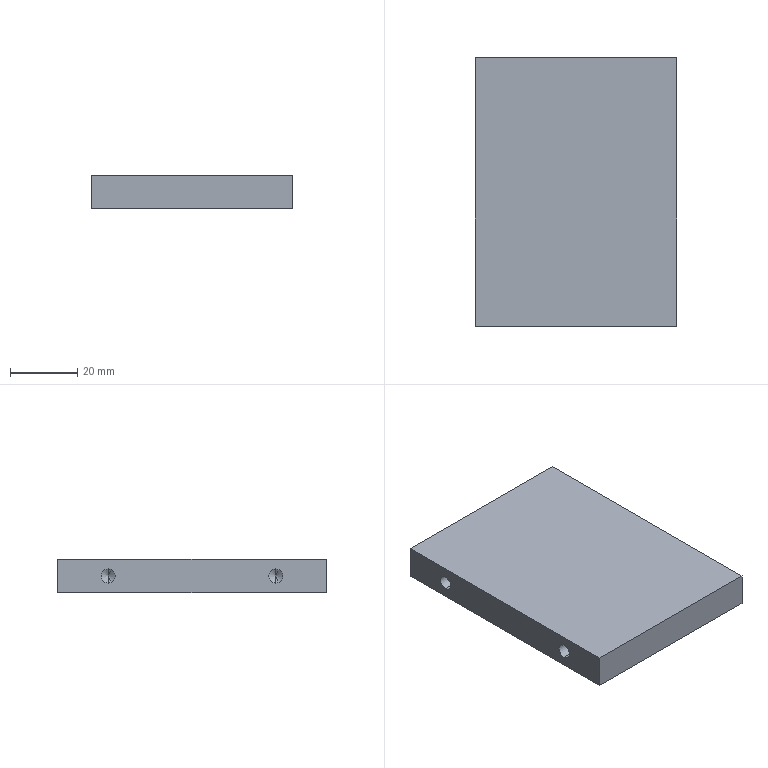Part | SolidWorks | features HoleWzd 2, Extrusion 1 | 1 solid | 22 faces | box 60 x 80 x 10 mm | volume 47201 mm3 | cylinder 8 | cone 8 | plane 6 | commonest cylinder face diameters 4.2 x8
STEP:
#1=CARTESIAN_POINT('',(-16.,25.,2.9));
#2=VERTEX_POINT('',#1);
#3=CARTESIAN_POINT('',(-16.,25.,7.1));
#4=VERTEX_POINT('',#3);
#5=CARTESIAN_POINT('',(-16.,25.,5.));
#6=DIRECTION('',(-1.,0.,0.));
#7=DIRECTION('',(0.,0.,1.));
#8=AXIS2_PLACEMENT_3D('',#5,#6,#7);
#9=CIRCLE('',#8,2.1);
#10=EDGE_CURVE('',#2,#4,#9,.T.);
#11=ORIENTED_EDGE('',*,*,#10,.F.);
#12=CARTESIAN_POINT('',(-30.,25.,2.9));
#13=VERTEX_POINT('',#12);
#14=CARTESIAN_POINT('',(-30.,25.,2.9));
#15=DIRECTION('',(-1.,0.,0.));
#16=VECTOR('',#15,1000.);
#17=LINE('',#14,#16);
#18=EDGE_CURVE('',#2,#13,#17,.T.);
#19=ORIENTED_EDGE('',*,*,#18,.T.);
#20=CARTESIAN_POINT('',(-30.,25.,7.1));
#21=VERTEX_POINT('',#20);
#22=CARTESIAN_POINT('',(-30.,25.,5.));
#23=DIRECTION('',(-1.,0.,0.));
#24=DIRECTION('',(0.,0.,1.));
#25=AXIS2_PLACEMENT_3D('',#22,#23,#24);
#26=CIRCLE('',#25,2.1);
#27=EDGE_CURVE('',#13,#21,#26,.T.);
#28=ORIENTED_EDGE('',*,*,#27,.T.);
#29=CARTESIAN_POINT('',(-30.,25.,7.1));
#30=DIRECTION('',(-1.,0.,0.));
#31=VECTOR('',#30,1000.);
#32=LINE('',#29,#31);
#33=EDGE_CURVE('',#4,#21,#32,.T.);
#34=ORIENTED_EDGE('',*,*,#33,.F.);
#35=EDGE_LOOP('',(#11,#19,#28,#34));
#36=FACE_OUTER_BOUND('',#35,.T.);
#37=CARTESIAN_POINT('',(-30.,25.,5.));
#38=DIRECTION('',(-1.,0.,0.));
#39=DIRECTION('',(0.,0.,1.));
#40=AXIS2_PLACEMENT_3D('',#37,#38,#39);
#41=CYLINDRICAL_SURFACE('',#40,2.1);
#42=ADVANCED_FACE('',(#36),#41,.F.);
#43=CARTESIAN_POINT('',(-14.738,25.,5.));
#44=VERTEX_POINT('',#43);
#45=CARTESIAN_POINT('',(-16.,25.,7.1));
#46=DIRECTION('',(-0.515,0.,0.8572));
#47=VECTOR('',#46,1000.);
#48=LINE('',#45,#47);
#49=EDGE_CURVE('',#44,#4,#48,.T.);
#50=ORIENTED_EDGE('',*,*,#49,.F.);
#51=CARTESIAN_POINT('',(-16.,25.,2.9));
#52=DIRECTION('',(-0.515,0.,-0.8572));
#53=VECTOR('',#52,1000.);
#54=LINE('',#51,#53);
#55=EDGE_CURVE('',#44,#2,#54,.T.);
#56=ORIENTED_EDGE('',*,*,#55,.T.);
#57=ORIENTED_EDGE('',*,*,#10,.T.);
#58=EDGE_LOOP('',(#50,#56,#57));
#59=FACE_OUTER_BOUND('',#58,.T.);
#60=CARTESIAN_POINT('',(-16.,25.,5.));
#61=DIRECTION('',(-1.,0.,0.));
#62=DIRECTION('',(0.,0.,1.));
#63=AXIS2_PLACEMENT_3D('',#60,#61,#62);
#64=CONICAL_SURFACE('',#63,2.1,1.03);
#65=ADVANCED_FACE('',(#59),#64,.F.);
#66=CARTESIAN_POINT('',(-16.,-25.,2.9));
#67=VERTEX_POINT('',#66);
#68=CARTESIAN_POINT('',(-16.,-25.,7.1));
#69=VERTEX_POINT('',#68);
#70=CARTESIAN_POINT('',(-16.,-25.,5.));
#71=DIRECTION('',(-1.,0.,0.));
#72=DIRECTION('',(0.,0.,1.));
#73=AXIS2_PLACEMENT_3D('',#70,#71,#72);
#74=CIRCLE('',#73,2.1);
#75=EDGE_CURVE('',#67,#69,#74,.T.);
#76=ORIENTED_EDGE('',*,*,#75,.F.);
#77=CARTESIAN_POINT('',(-30.,-25.,2.9));
#78=VERTEX_POINT('',#77);
#79=CARTESIAN_POINT('',(-30.,-25.,2.9));
#80=DIRECTION('',(-1.,0.,0.));
#81=VECTOR('',#80,1000.);
#82=LINE('',#79,#81);
#83=EDGE_CURVE('',#67,#78,#82,.T.);
#84=ORIENTED_EDGE('',*,*,#83,.T.);
#85=CARTESIAN_POINT('',(-30.,-25.,7.1));
#86=VERTEX_POINT('',#85);
#87=CARTESIAN_POINT('',(-30.,-25.,5.));
#88=DIRECTION('',(-1.,0.,0.));
#89=DIRECTION('',(0.,0.,1.));
#90=AXIS2_PLACEMENT_3D('',#87,#88,#89);
#91=CIRCLE('',#90,2.1);
#92=EDGE_CURVE('',#78,#86,#91,.T.);
#93=ORIENTED_EDGE('',*,*,#92,.T.);
#94=CARTESIAN_POINT('',(-30.,-25.,7.1));
#95=DIRECTION('',(-1.,0.,0.));
#96=VECTOR('',#95,1000.);
#97=LINE('',#94,#96);
#98=EDGE_CURVE('',#69,#86,#97,.T.);
#99=ORIENTED_EDGE('',*,*,#98,.F.);
#100=EDGE_LOOP('',(#76,#84,#93,#99));
#101=FACE_OUTER_BOUND('',#100,.T.);
#102=CARTESIAN_POINT('',(-30.,-25.,5.));
#103=DIRECTION('',(-1.,0.,0.));
#104=DIRECTION('',(0.,0.,1.));
#105=AXIS2_PLACEMENT_3D('',#102,#103,#104);
#106=CYLINDRICAL_SURFACE('',#105,2.1);
#107=ADVANCED_FACE('',(#101),#106,.F.);
#108=CARTESIAN_POINT('',(-14.738,-25.,5.));
#109=VERTEX_POINT('',#108);
#110=CARTESIAN_POINT('',(-16.,-25.,7.1));
#111=DIRECTION('',(-0.515,0.,0.8572));
#112=VECTOR('',#111,1000.);
#113=LINE('',#110,#112);
#114=EDGE_CURVE('',#109,#69,#113,.T.);
#115=ORIENTED_EDGE('',*,*,#114,.F.);
#116=CARTESIAN_POINT('',(-16.,-25.,2.9));
#117=DIRECTION('',(-0.515,0.,-0.8572));
#118=VECTOR('',#117,1000.);
#119=LINE('',#116,#118);
#120=EDGE_CURVE('',#109,#67,#119,.T.);
#121=ORIENTED_EDGE('',*,*,#120,.T.);
#122=ORIENTED_EDGE('',*,*,#75,.T.);
#123=EDGE_LOOP('',(#115,#121,#122));
#124=FACE_OUTER_BOUND('',#123,.T.);
#125=CARTESIAN_POINT('',(-16.,-25.,5.));
#126=DIRECTION('',(-1.,0.,0.));
#127=DIRECTION('',(0.,0.,1.));
#128=AXIS2_PLACEMENT_3D('',#125,#126,#127);
#129=CONICAL_SURFACE('',#128,2.1,1.03);
#130=ADVANCED_FACE('',(#124),#129,.F.);
#131=CARTESIAN_POINT('',(16.,-25.,7.1));
#132=VERTEX_POINT('',#131);
#133=CARTESIAN_POINT('',(16.,-25.,2.9));
#134=VERTEX_POINT('',#133);
#135=CARTESIAN_POINT('',(16.,-25.,5.));
#136=DIRECTION('',(1.,0.,0.));
#137=DIRECTION('',(0.,0.,-1.));
#138=AXIS2_PLACEMENT_3D('',#135,#136,#137);
#139=CIRCLE('',#138,2.1);
#140=EDGE_CURVE('',#132,#134,#139,.T.);
#141=ORIENTED_EDGE('',*,*,#140,.F.);
#142=CARTESIAN_POINT('',(30.,-25.,7.1));
#143=VERTEX_POINT('',#142);
#144=CARTESIAN_POINT('',(30.,-25.,7.1));
#145=DIRECTION('',(1.,0.,0.));
#146=VECTOR('',#145,1000.);
#147=LINE('',#144,#146);
#148=EDGE_CURVE('',#132,#143,#147,.T.);
#149=ORIENTED_EDGE('',*,*,#148,.T.);
#150=CARTESIAN_POINT('',(30.,-25.,2.9));
#151=VERTEX_POINT('',#150);
#152=CARTESIAN_POINT('',(30.,-25.,5.));
#153=DIRECTION('',(1.,0.,0.));
#154=DIRECTION('',(0.,0.,-1.));
#155=AXIS2_PLACEMENT_3D('',#152,#153,#154);
#156=CIRCLE('',#155,2.1);
#157=EDGE_CURVE('',#143,#151,#156,.T.);
#158=ORIENTED_EDGE('',*,*,#157,.T.);
#159=CARTESIAN_POINT('',(30.,-25.,2.9));
#160=DIRECTION('',(1.,0.,0.));
#161=VECTOR('',#160,1000.);
#162=LINE('',#159,#161);
#163=EDGE_CURVE('',#134,#151,#162,.T.);
#164=ORIENTED_EDGE('',*,*,#163,.F.);
#165=EDGE_LOOP('',(#141,#149,#158,#164));
#166=FACE_OUTER_BOUND('',#165,.T.);
#167=CARTESIAN_POINT('',(30.,-25.,5.));
#168=DIRECTION('',(1.,0.,0.));
#169=DIRECTION('',(0.,0.,-1.));
#170=AXIS2_PLACEMENT_3D('',#167,#168,#169);
#171=CYLINDRICAL_SURFACE('',#170,2.1);
#172=ADVANCED_FACE('',(#166),#171,.F.);
#173=CARTESIAN_POINT('',(14.738,-25.,5.));
#174=VERTEX_POINT('',#173);
#175=CARTESIAN_POINT('',(16.,-25.,2.9));
#176=DIRECTION('',(0.515,0.,-0.8572));
#177=VECTOR('',#176,1000.);
#178=LINE('',#175,#177);
#179=EDGE_CURVE('',#174,#134,#178,.T.);
#180=ORIENTED_EDGE('',*,*,#179,.F.);
#181=CARTESIAN_POINT('',(16.,-25.,7.1));
#182=DIRECTION('',(0.515,0.,0.8572));
#183=VECTOR('',#182,1000.);
#184=LINE('',#181,#183);
#185=EDGE_CURVE('',#174,#132,#184,.T.);
#186=ORIENTED_EDGE('',*,*,#185,.T.);
#187=ORIENTED_EDGE('',*,*,#140,.T.);
#188=EDGE_LOOP('',(#180,#186,#187));
#189=FACE_OUTER_BOUND('',#188,.T.);
#190=CARTESIAN_POINT('',(16.,-25.,5.));
#191=DIRECTION('',(1.,0.,0.));
#192=DIRECTION('',(0.,0.,-1.));
#193=AXIS2_PLACEMENT_3D('',#190,#191,#192);
#194=CONICAL_SURFACE('',#193,2.1,1.03);
#195=ADVANCED_FACE('',(#189),#194,.F.);
#196=CARTESIAN_POINT('',(16.,25.,7.1));
#197=VERTEX_POINT('',#196);
#198=CARTESIAN_POINT('',(16.,25.,2.9));
#199=VERTEX_POINT('',#198);
#200=CARTESIAN_POINT('',(16.,25.,5.));
#201=DIRECTION('',(1.,0.,0.));
#202=DIRECTION('',(0.,0.,-1.));
#203=AXIS2_PLACEMENT_3D('',#200,#201,#202);
#204=CIRCLE('',#203,2.1);
#205=EDGE_CURVE('',#197,#199,#204,.T.);
#206=ORIENTED_EDGE('',*,*,#205,.F.);
#207=CARTESIAN_POINT('',(30.,25.,7.1));
#208=VERTEX_POINT('',#207);
#209=CARTESIAN_POINT('',(30.,25.,7.1));
#210=DIRECTION('',(1.,0.,0.));
#211=VECTOR('',#210,1000.);
#212=LINE('',#209,#211);
#213=EDGE_CURVE('',#197,#208,#212,.T.);
#214=ORIENTED_EDGE('',*,*,#213,.T.);
#215=CARTESIAN_POINT('',(30.,25.,2.9));
#216=VERTEX_POINT('',#215);
#217=CARTESIAN_POINT('',(30.,25.,5.));
#218=DIRECTION('',(1.,0.,0.));
#219=DIRECTION('',(0.,0.,-1.));
#220=AXIS2_PLACEMENT_3D('',#217,#218,#219);
#221=CIRCLE('',#220,2.1);
#222=EDGE_CURVE('',#208,#216,#221,.T.);
#223=ORIENTED_EDGE('',*,*,#222,.T.);
#224=CARTESIAN_POINT('',(30.,25.,2.9));
#225=DIRECTION('',(1.,0.,0.));
#226=VECTOR('',#225,1000.);
#227=LINE('',#224,#226);
#228=EDGE_CURVE('',#199,#216,#227,.T.);
#229=ORIENTED_EDGE('',*,*,#228,.F.);
#230=EDGE_LOOP('',(#206,#214,#223,#229));
#231=FACE_OUTER_BOUND('',#230,.T.);
#232=CARTESIAN_POINT('',(30.,25.,5.));
#233=DIRECTION('',(1.,0.,0.));
#234=DIRECTION('',(0.,0.,-1.));
#235=AXIS2_PLACEMENT_3D('',#232,#233,#234);
#236=CYLINDRICAL_SURFACE('',#235,2.1);
#237=ADVANCED_FACE('',(#231),#236,.F.);
#238=CARTESIAN_POINT('',(14.738,25.,5.));
#239=VERTEX_POINT('',#238);
#240=CARTESIAN_POINT('',(16.,25.,2.9));
#241=DIRECTION('',(0.515,0.,-0.8572));
#242=VECTOR('',#241,1000.);
#243=LINE('',#240,#242);
#244=EDGE_CURVE('',#239,#199,#243,.T.);
#245=ORIENTED_EDGE('',*,*,#244,.F.);
#246=CARTESIAN_POINT('',(16.,25.,7.1));
#247=DIRECTION('',(0.515,0.,0.8572));
#248=VECTOR('',#247,1000.);
#249=LINE('',#246,#248);
#250=EDGE_CURVE('',#239,#197,#249,.T.);
#251=ORIENTED_EDGE('',*,*,#250,.T.);
#252=ORIENTED_EDGE('',*,*,#205,.T.);
#253=EDGE_LOOP('',(#245,#251,#252));
#254=FACE_OUTER_BOUND('',#253,.T.);
#255=CARTESIAN_POINT('',(16.,25.,5.));
#256=DIRECTION('',(1.,0.,0.));
#257=DIRECTION('',(0.,0.,-1.));
#258=AXIS2_PLACEMENT_3D('',#255,#256,#257);
#259=CONICAL_SURFACE('',#258,2.1,1.03);
#260=ADVANCED_FACE('',(#254),#259,.F.);
#261=CARTESIAN_POINT('',(30.,-25.,5.));
#262=DIRECTION('',(1.,0.,0.));
#263=DIRECTION('',(0.,0.,-1.));
#264=AXIS2_PLACEMENT_3D('',#261,#262,#263);
#265=CIRCLE('',#264,2.1);
#266=EDGE_CURVE('',#151,#143,#265,.T.);
#267=ORIENTED_EDGE('',*,*,#266,.F.);
#268=ORIENTED_EDGE('',*,*,#157,.F.);
#269=EDGE_LOOP('',(#267,#268));
#270=FACE_BOUND('',#269,.T.);
#271=CARTESIAN_POINT('',(30.,25.,5.));
#272=DIRECTION('',(1.,0.,0.));
#273=DIRECTION('',(0.,0.,-1.));
#274=AXIS2_PLACEMENT_3D('',#271,#272,#273);
#275=CIRCLE('',#274,2.1);
#276=EDGE_CURVE('',#216,#208,#275,.T.);
#277=ORIENTED_EDGE('',*,*,#276,.F.);
#278=ORIENTED_EDGE('',*,*,#222,.F.);
#279=EDGE_LOOP('',(#277,#278));
#280=FACE_BOUND('',#279,.T.);
#281=CARTESIAN_POINT('',(30.,-40.,0.));
#282=VERTEX_POINT('',#281);
#283=CARTESIAN_POINT('',(30.,40.,0.));
#284=VERTEX_POINT('',#283);
#285=CARTESIAN_POINT('',(30.,40.,0.));
#286=DIRECTION('',(0.,1.,0.));
#287=VECTOR('',#286,1000.);
#288=LINE('',#285,#287);
#289=EDGE_CURVE('',#282,#284,#288,.T.);
#290=ORIENTED_EDGE('',*,*,#289,.T.);
#291=CARTESIAN_POINT('',(30.,40.,10.));
#292=VERTEX_POINT('',#291);
#293=CARTESIAN_POINT('',(30.,40.,10.));
#294=DIRECTION('',(0.,0.,-1.));
#295=VECTOR('',#294,1000.);
#296=LINE('',#293,#295);
#297=EDGE_CURVE('',#292,#284,#296,.T.);
#298=ORIENTED_EDGE('',*,*,#297,.F.);
#299=CARTESIAN_POINT('',(30.,-40.,10.));
#300=VERTEX_POINT('',#299);
#301=CARTESIAN_POINT('',(30.,40.,10.));
#302=DIRECTION('',(0.,1.,0.));
#303=VECTOR('',#302,1000.);
#304=LINE('',#301,#303);
#305=EDGE_CURVE('',#300,#292,#304,.T.);
#306=ORIENTED_EDGE('',*,*,#305,.F.);
#307=CARTESIAN_POINT('',(30.,-40.,10.));
#308=DIRECTION('',(0.,0.,-1.));
#309=VECTOR('',#308,1000.);
#310=LINE('',#307,#309);
#311=EDGE_CURVE('',#300,#282,#310,.T.);
#312=ORIENTED_EDGE('',*,*,#311,.T.);
#313=EDGE_LOOP('',(#290,#298,#306,#312));
#314=FACE_OUTER_BOUND('',#313,.T.);
#315=CARTESIAN_POINT('',(30.,40.,10.));
#316=DIRECTION('',(-1.,0.,0.));
#317=DIRECTION('',(0.,-1.,0.));
#318=AXIS2_PLACEMENT_3D('',#315,#316,#317);
#319=PLANE('',#318);
#320=ADVANCED_FACE('',(#270,#280,#314),#319,.F.);
#321=CARTESIAN_POINT('',(-30.,40.,0.));
#322=VERTEX_POINT('',#321);
#323=CARTESIAN_POINT('',(-30.,40.,0.));
#324=DIRECTION('',(-1.,0.,0.));
#325=VECTOR('',#324,1000.);
#326=LINE('',#323,#325);
#327=EDGE_CURVE('',#284,#322,#326,.T.);
#328=ORIENTED_EDGE('',*,*,#327,.T.);
#329=CARTESIAN_POINT('',(-30.,40.,10.));
#330=VERTEX_POINT('',#329);
#331=CARTESIAN_POINT('',(-30.,40.,10.));
#332=DIRECTION('',(0.,0.,-1.));
#333=VECTOR('',#332,1000.);
#334=LINE('',#331,#333);
#335=EDGE_CURVE('',#330,#322,#334,.T.);
#336=ORIENTED_EDGE('',*,*,#335,.F.);
#337=CARTESIAN_POINT('',(-30.,40.,10.));
#338=DIRECTION('',(-1.,0.,0.));
#339=VECTOR('',#338,1000.);
#340=LINE('',#337,#339);
#341=EDGE_CURVE('',#292,#330,#340,.T.);
#342=ORIENTED_EDGE('',*,*,#341,.F.);
#343=ORIENTED_EDGE('',*,*,#297,.T.);
#344=EDGE_LOOP('',(#328,#336,#342,#343));
#345=FACE_OUTER_BOUND('',#344,.T.);
#346=CARTESIAN_POINT('',(-30.,40.,10.));
#347=DIRECTION('',(0.,-1.,0.));
#348=DIRECTION('',(0.,0.,-1.));
#349=AXIS2_PLACEMENT_3D('',#346,#347,#348);
#350=PLANE('',#349);
#351=ADVANCED_FACE('',(#345),#350,.F.);
#352=CARTESIAN_POINT('',(-30.,25.,5.));
#353=DIRECTION('',(-1.,0.,0.));
#354=DIRECTION('',(0.,0.,1.));
#355=AXIS2_PLACEMENT_3D('',#352,#353,#354);
#356=CIRCLE('',#355,2.1);
#357=EDGE_CURVE('',#21,#13,#356,.T.);
#358=ORIENTED_EDGE('',*,*,#357,.F.);
#359=ORIENTED_EDGE('',*,*,#27,.F.);
#360=EDGE_LOOP('',(#358,#359));
#361=FACE_BOUND('',#360,.T.);
#362=CARTESIAN_POINT('',(-30.,-25.,5.));
#363=DIRECTION('',(-1.,0.,0.));
#364=DIRECTION('',(0.,0.,1.));
#365=AXIS2_PLACEMENT_3D('',#362,#363,#364);
#366=CIRCLE('',#365,2.1);
#367=EDGE_CURVE('',#86,#78,#366,.T.);
#368=ORIENTED_EDGE('',*,*,#367,.F.);
#369=ORIENTED_EDGE('',*,*,#92,.F.);
#370=EDGE_LOOP('',(#368,#369));
#371=FACE_BOUND('',#370,.T.);
#372=CARTESIAN_POINT('',(-30.,-40.,0.));
#373=VERTEX_POINT('',#372);
#374=CARTESIAN_POINT('',(-30.,40.,0.));
#375=DIRECTION('',(0.,-1.,0.));
#376=VECTOR('',#375,1000.);
#377=LINE('',#374,#376);
#378=EDGE_CURVE('',#322,#373,#377,.T.);
#379=ORIENTED_EDGE('',*,*,#378,.T.);
#380=CARTESIAN_POINT('',(-30.,-40.,10.));
#381=VERTEX_POINT('',#380);
#382=CARTESIAN_POINT('',(-30.,-40.,10.));
#383=DIRECTION('',(0.,0.,-1.));
#384=VECTOR('',#383,1000.);
#385=LINE('',#382,#384);
#386=EDGE_CURVE('',#381,#373,#385,.T.);
#387=ORIENTED_EDGE('',*,*,#386,.F.);
#388=CARTESIAN_POINT('',(-30.,40.,10.));
#389=DIRECTION('',(0.,-1.,0.));
#390=VECTOR('',#389,1000.);
#391=LINE('',#388,#390);
#392=EDGE_CURVE('',#330,#381,#391,.T.);
#393=ORIENTED_EDGE('',*,*,#392,.F.);
#394=ORIENTED_EDGE('',*,*,#335,.T.);
#395=EDGE_LOOP('',(#379,#387,#393,#394));
#396=FACE_OUTER_BOUND('',#395,.T.);
#397=CARTESIAN_POINT('',(-30.,40.,10.));
#398=DIRECTION('',(1.,0.,0.));
#399=DIRECTION('',(0.,1.,0.));
#400=AXIS2_PLACEMENT_3D('',#397,#398,#399);
#401=PLANE('',#400);
#402=ADVANCED_FACE('',(#361,#371,#396),#401,.F.);
#403=CARTESIAN_POINT('',(-30.,-40.,0.));
#404=DIRECTION('',(1.,0.,0.));
#405=VECTOR('',#404,1000.);
#406=LINE('',#403,#405);
#407=EDGE_CURVE('',#373,#282,#406,.T.);
#408=ORIENTED_EDGE('',*,*,#407,.T.);
#409=ORIENTED_EDGE('',*,*,#311,.F.);
#410=CARTESIAN_POINT('',(-30.,-40.,10.));
#411=DIRECTION('',(1.,0.,0.));
#412=VECTOR('',#411,1000.);
#413=LINE('',#410,#412);
#414=EDGE_CURVE('',#381,#300,#413,.T.);
#415=ORIENTED_EDGE('',*,*,#414,.F.);
#416=ORIENTED_EDGE('',*,*,#386,.T.);
#417=EDGE_LOOP('',(#408,#409,#415,#416));
#418=FACE_OUTER_BOUND('',#417,.T.);
#419=CARTESIAN_POINT('',(-30.,-40.,10.));
#420=DIRECTION('',(0.,1.,0.));
#421=DIRECTION('',(0.,0.,1.));
#422=AXIS2_PLACEMENT_3D('',#419,#420,#421);
#423=PLANE('',#422);
#424=ADVANCED_FACE('',(#418),#423,.F.);
#425=ORIENTED_EDGE('',*,*,#305,.T.);
#426=ORIENTED_EDGE('',*,*,#341,.T.);
#427=ORIENTED_EDGE('',*,*,#392,.T.);
#428=ORIENTED_EDGE('',*,*,#414,.T.);
#429=EDGE_LOOP('',(#425,#426,#427,#428));
#430=FACE_OUTER_BOUND('',#429,.T.);
#431=CARTESIAN_POINT('',(0.,0.,10.));
#432=DIRECTION('',(0.,0.,1.));
#433=DIRECTION('',(1.,0.,0.));
#434=AXIS2_PLACEMENT_3D('',#431,#432,#433);
#435=PLANE('',#434);
#436=ADVANCED_FACE('',(#430),#435,.T.);
#437=ORIENTED_EDGE('',*,*,#289,.F.);
#438=ORIENTED_EDGE('',*,*,#407,.F.);
#439=ORIENTED_EDGE('',*,*,#378,.F.);
#440=ORIENTED_EDGE('',*,*,#327,.F.);
#441=EDGE_LOOP('',(#437,#438,#439,#440));
#442=FACE_OUTER_BOUND('',#441,.T.);
#443=CARTESIAN_POINT('',(0.,0.,0.));
#444=DIRECTION('',(0.,0.,1.));
#445=DIRECTION('',(1.,0.,0.));
#446=AXIS2_PLACEMENT_3D('',#443,#444,#445);
#447=PLANE('',#446);
#448=ADVANCED_FACE('',(#442),#447,.F.);
#449=ORIENTED_EDGE('',*,*,#250,.F.);
#450=ORIENTED_EDGE('',*,*,#244,.T.);
#451=CARTESIAN_POINT('',(16.,25.,5.));
#452=DIRECTION('',(1.,0.,0.));
#453=DIRECTION('',(0.,0.,-1.));
#454=AXIS2_PLACEMENT_3D('',#451,#452,#453);
#455=CIRCLE('',#454,2.1);
#456=EDGE_CURVE('',#199,#197,#455,.T.);
#457=ORIENTED_EDGE('',*,*,#456,.T.);
#458=EDGE_LOOP('',(#449,#450,#457));
#459=FACE_OUTER_BOUND('',#458,.T.);
#460=CARTESIAN_POINT('',(16.,25.,5.));
#461=DIRECTION('',(1.,0.,0.));
#462=DIRECTION('',(0.,0.,-1.));
#463=AXIS2_PLACEMENT_3D('',#460,#461,#462);
#464=CONICAL_SURFACE('',#463,2.1,1.03);
#465=ADVANCED_FACE('',(#459),#464,.F.);
#466=ORIENTED_EDGE('',*,*,#213,.F.);
#467=ORIENTED_EDGE('',*,*,#456,.F.);
#468=ORIENTED_EDGE('',*,*,#228,.T.);
#469=ORIENTED_EDGE('',*,*,#276,.T.);
#470=EDGE_LOOP('',(#466,#467,#468,#469));
#471=FACE_OUTER_BOUND('',#470,.T.);
#472=CARTESIAN_POINT('',(30.,25.,5.));
#473=DIRECTION('',(1.,0.,0.));
#474=DIRECTION('',(0.,0.,-1.));
#475=AXIS2_PLACEMENT_3D('',#472,#473,#474);
#476=CYLINDRICAL_SURFACE('',#475,2.1);
#477=ADVANCED_FACE('',(#471),#476,.F.);
#478=ORIENTED_EDGE('',*,*,#185,.F.);
#479=ORIENTED_EDGE('',*,*,#179,.T.);
#480=CARTESIAN_POINT('',(16.,-25.,5.));
#481=DIRECTION('',(1.,0.,0.));
#482=DIRECTION('',(0.,0.,-1.));
#483=AXIS2_PLACEMENT_3D('',#480,#481,#482);
#484=CIRCLE('',#483,2.1);
#485=EDGE_CURVE('',#134,#132,#484,.T.);
#486=ORIENTED_EDGE('',*,*,#485,.T.);
#487=EDGE_LOOP('',(#478,#479,#486));
#488=FACE_OUTER_BOUND('',#487,.T.);
#489=CARTESIAN_POINT('',(16.,-25.,5.));
#490=DIRECTION('',(1.,0.,0.));
#491=DIRECTION('',(0.,0.,-1.));
#492=AXIS2_PLACEMENT_3D('',#489,#490,#491);
#493=CONICAL_SURFACE('',#492,2.1,1.03);
#494=ADVANCED_FACE('',(#488),#493,.F.);
#495=ORIENTED_EDGE('',*,*,#148,.F.);
#496=ORIENTED_EDGE('',*,*,#485,.F.);
#497=ORIENTED_EDGE('',*,*,#163,.T.);
#498=ORIENTED_EDGE('',*,*,#266,.T.);
#499=EDGE_LOOP('',(#495,#496,#497,#498));
#500=FACE_OUTER_BOUND('',#499,.T.);
#501=CARTESIAN_POINT('',(30.,-25.,5.));
#502=DIRECTION('',(1.,0.,0.));
#503=DIRECTION('',(0.,0.,-1.));
#504=AXIS2_PLACEMENT_3D('',#501,#502,#503);
#505=CYLINDRICAL_SURFACE('',#504,2.1);
#506=ADVANCED_FACE('',(#500),#505,.F.);
#507=ORIENTED_EDGE('',*,*,#120,.F.);
#508=ORIENTED_EDGE('',*,*,#114,.T.);
#509=CARTESIAN_POINT('',(-16.,-25.,5.));
#510=DIRECTION('',(-1.,0.,0.));
#511=DIRECTION('',(0.,0.,1.));
#512=AXIS2_PLACEMENT_3D('',#509,#510,#511);
#513=CIRCLE('',#512,2.1);
#514=EDGE_CURVE('',#69,#67,#513,.T.);
#515=ORIENTED_EDGE('',*,*,#514,.T.);
#516=EDGE_LOOP('',(#507,#508,#515));
#517=FACE_OUTER_BOUND('',#516,.T.);
#518=CARTESIAN_POINT('',(-16.,-25.,5.));
#519=DIRECTION('',(-1.,0.,0.));
#520=DIRECTION('',(0.,0.,1.));
#521=AXIS2_PLACEMENT_3D('',#518,#519,#520);
#522=CONICAL_SURFACE('',#521,2.1,1.03);
#523=ADVANCED_FACE('',(#517),#522,.F.);
#524=ORIENTED_EDGE('',*,*,#83,.F.);
#525=ORIENTED_EDGE('',*,*,#514,.F.);
#526=ORIENTED_EDGE('',*,*,#98,.T.);
#527=ORIENTED_EDGE('',*,*,#367,.T.);
#528=EDGE_LOOP('',(#524,#525,#526,#527));
#529=FACE_OUTER_BOUND('',#528,.T.);
#530=CARTESIAN_POINT('',(-30.,-25.,5.));
#531=DIRECTION('',(-1.,0.,0.));
#532=DIRECTION('',(0.,0.,1.));
#533=AXIS2_PLACEMENT_3D('',#530,#531,#532);
#534=CYLINDRICAL_SURFACE('',#533,2.1);
#535=ADVANCED_FACE('',(#529),#534,.F.);
#536=ORIENTED_EDGE('',*,*,#55,.F.);
#537=ORIENTED_EDGE('',*,*,#49,.T.);
#538=CARTESIAN_POINT('',(-16.,25.,5.));
#539=DIRECTION('',(-1.,0.,0.));
#540=DIRECTION('',(0.,0.,1.));
#541=AXIS2_PLACEMENT_3D('',#538,#539,#540);
#542=CIRCLE('',#541,2.1);
#543=EDGE_CURVE('',#4,#2,#542,.T.);
#544=ORIENTED_EDGE('',*,*,#543,.T.);
#545=EDGE_LOOP('',(#536,#537,#544));
#546=FACE_OUTER_BOUND('',#545,.T.);
#547=CARTESIAN_POINT('',(-16.,25.,5.));
#548=DIRECTION('',(-1.,0.,0.));
#549=DIRECTION('',(0.,0.,1.));
#550=AXIS2_PLACEMENT_3D('',#547,#548,#549);
#551=CONICAL_SURFACE('',#550,2.1,1.03);
#552=ADVANCED_FACE('',(#546),#551,.F.);
#553=ORIENTED_EDGE('',*,*,#18,.F.);
#554=ORIENTED_EDGE('',*,*,#543,.F.);
#555=ORIENTED_EDGE('',*,*,#33,.T.);
#556=ORIENTED_EDGE('',*,*,#357,.T.);
#557=EDGE_LOOP('',(#553,#554,#555,#556));
#558=FACE_OUTER_BOUND('',#557,.T.);
#559=CARTESIAN_POINT('',(-30.,25.,5.));
#560=DIRECTION('',(-1.,0.,0.));
#561=DIRECTION('',(0.,0.,1.));
#562=AXIS2_PLACEMENT_3D('',#559,#560,#561);
#563=CYLINDRICAL_SURFACE('',#562,2.1);
#564=ADVANCED_FACE('',(#558),#563,.F.);
#565=CLOSED_SHELL('',(#42,#65,#107,#130,#172,#195,#237,#260,#320,#351,#402,#424,#436,#448,#465,#477,#494,#506,#523,#535,#552,#564));
#566=MANIFOLD_SOLID_BREP('',#565);
#567=CARTESIAN_POINT('',(0.,0.,0.));
#568=DIRECTION('',(0.,0.,1.));
#569=DIRECTION('',(1.,0.,0.));
#570=AXIS2_PLACEMENT_3D('',#567,#568,#569);
#571=(LENGTH_UNIT()NAMED_UNIT(*)SI_UNIT(.MILLI.,.METRE.));
#572=UNCERTAINTY_MEASURE_WITH_UNIT(LENGTH_MEASURE(0.00001),#571,'','');
#573=(NAMED_UNIT(*)PLANE_ANGLE_UNIT()SI_UNIT($,.RADIAN.));
#574=(NAMED_UNIT(*)SI_UNIT($,.STERADIAN.)SOLID_ANGLE_UNIT());
#575=(GEOMETRIC_REPRESENTATION_CONTEXT(3)GLOBAL_UNCERTAINTY_ASSIGNED_CONTEXT((#572))GLOBAL_UNIT_ASSIGNED_CONTEXT((#571,#573,#574))REPRESENTATION_CONTEXT('',''));
#576=ADVANCED_BREP_SHAPE_REPRESENTATION('',(#566,#570),#575);